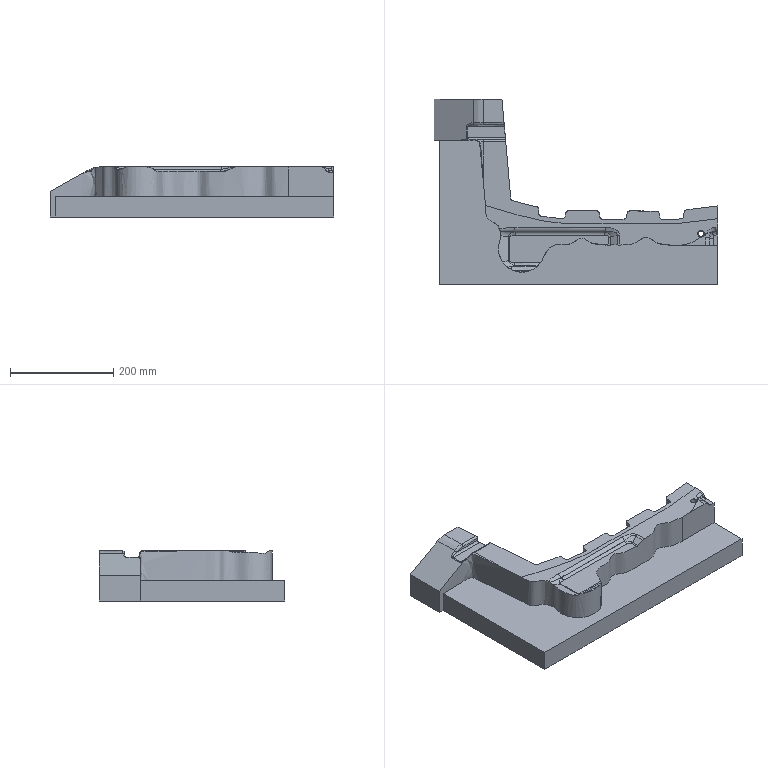Part | NX | features solid 2 | 1 solid | 82 faces | box 550 x 360 x 97 mm | volume 5944260 mm3 | spline 74 | plane 6 | cylinder 2 | commonest cylinder face diameters 10.4 x1 13 x1